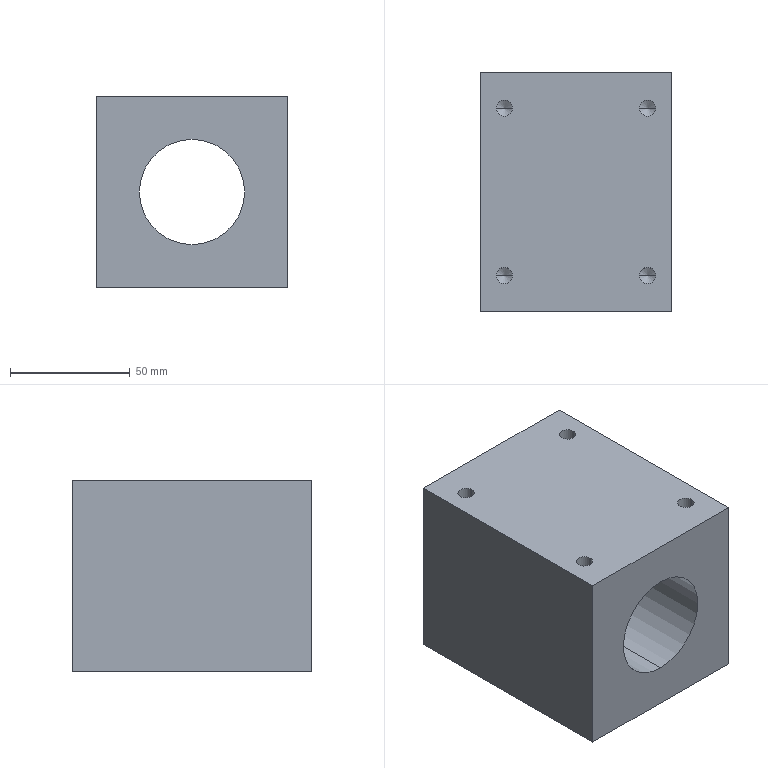Part | SolidWorks | features BaseBody 1 | 1 solid | 48 faces | box 80 x 100 x 80 mm | volume 483153 mm3 | cylinder 22 | cone 20 | plane 6 | commonest cylinder face diameters 5 x12 6.8 x8 44 x2
STEP:
#1=CARTESIAN_POINT('',(-66.6,85.,60.25));
#2=VERTEX_POINT('',#1);
#3=CARTESIAN_POINT('',(-73.4,85.,60.25));
#4=VERTEX_POINT('',#3);
#5=CARTESIAN_POINT('',(-70.,85.,60.25));
#6=DIRECTION('',(0.,0.,-1.));
#7=DIRECTION('',(1.,0.,0.));
#8=AXIS2_PLACEMENT_3D('',#5,#6,#7);
#9=CIRCLE('',#8,3.4);
#10=EDGE_CURVE('',#2,#4,#9,.T.);
#11=ORIENTED_EDGE('',*,*,#10,.T.);
#12=CARTESIAN_POINT('',(-73.4,85.,80.));
#13=VERTEX_POINT('',#12);
#14=CARTESIAN_POINT('',(-73.4,85.,60.25));
#15=DIRECTION('',(0.,0.,1.));
#16=VECTOR('',#15,1000.);
#17=LINE('',#14,#16);
#18=EDGE_CURVE('',#4,#13,#17,.T.);
#19=ORIENTED_EDGE('',*,*,#18,.T.);
#20=CARTESIAN_POINT('',(-66.6,85.,80.));
#21=VERTEX_POINT('',#20);
#22=CARTESIAN_POINT('',(-70.,85.,80.));
#23=DIRECTION('',(0.,0.,1.));
#24=DIRECTION('',(1.,0.,0.));
#25=AXIS2_PLACEMENT_3D('',#22,#23,#24);
#26=CIRCLE('',#25,3.4);
#27=EDGE_CURVE('',#13,#21,#26,.T.);
#28=ORIENTED_EDGE('',*,*,#27,.T.);
#29=CARTESIAN_POINT('',(-66.6,85.,60.25));
#30=DIRECTION('',(0.,0.,1.));
#31=VECTOR('',#30,1000.);
#32=LINE('',#29,#31);
#33=EDGE_CURVE('',#2,#21,#32,.T.);
#34=ORIENTED_EDGE('',*,*,#33,.F.);
#35=EDGE_LOOP('',(#11,#19,#28,#34));
#36=FACE_OUTER_BOUND('',#35,.T.);
#37=CARTESIAN_POINT('',(-70.,85.,60.25));
#38=DIRECTION('',(0.,0.,1.));
#39=DIRECTION('',(1.,0.,0.));
#40=AXIS2_PLACEMENT_3D('',#37,#38,#39);
#41=CYLINDRICAL_SURFACE('',#40,3.4);
#42=ADVANCED_FACE('',(#36),#41,.F.);
#43=CARTESIAN_POINT('',(-70.,85.,58.207));
#44=VERTEX_POINT('',#43);
#45=CARTESIAN_POINT('',(-70.,85.,58.207));
#46=DIRECTION('',(0.8572,0.,0.515));
#47=VECTOR('',#46,1000.);
#48=LINE('',#45,#47);
#49=EDGE_CURVE('',#44,#2,#48,.T.);
#50=ORIENTED_EDGE('',*,*,#49,.F.);
#51=CARTESIAN_POINT('',(-70.,85.,58.207));
#52=DIRECTION('',(-0.8572,0.,0.515));
#53=VECTOR('',#52,1000.);
#54=LINE('',#51,#53);
#55=EDGE_CURVE('',#44,#4,#54,.T.);
#56=ORIENTED_EDGE('',*,*,#55,.T.);
#57=ORIENTED_EDGE('',*,*,#10,.F.);
#58=EDGE_LOOP('',(#50,#56,#57));
#59=FACE_OUTER_BOUND('',#58,.T.);
#60=CARTESIAN_POINT('',(-70.,85.,1058.207));
#61=DIRECTION('',(0.,0.,1.));
#62=DIRECTION('',(1.,0.,0.));
#63=AXIS2_PLACEMENT_3D('',#60,#61,#62);
#64=CONICAL_SURFACE('',#63,1664.279,1.03);
#65=ADVANCED_FACE('',(#59),#64,.F.);
#66=CARTESIAN_POINT('',(-6.6,85.,60.25));
#67=VERTEX_POINT('',#66);
#68=CARTESIAN_POINT('',(-13.4,85.,60.25));
#69=VERTEX_POINT('',#68);
#70=CARTESIAN_POINT('',(-10.,85.,60.25));
#71=DIRECTION('',(0.,0.,-1.));
#72=DIRECTION('',(1.,0.,0.));
#73=AXIS2_PLACEMENT_3D('',#70,#71,#72);
#74=CIRCLE('',#73,3.4);
#75=EDGE_CURVE('',#67,#69,#74,.T.);
#76=ORIENTED_EDGE('',*,*,#75,.T.);
#77=CARTESIAN_POINT('',(-13.4,85.,80.));
#78=VERTEX_POINT('',#77);
#79=CARTESIAN_POINT('',(-13.4,85.,60.25));
#80=DIRECTION('',(0.,0.,1.));
#81=VECTOR('',#80,1000.);
#82=LINE('',#79,#81);
#83=EDGE_CURVE('',#69,#78,#82,.T.);
#84=ORIENTED_EDGE('',*,*,#83,.T.);
#85=CARTESIAN_POINT('',(-6.6,85.,80.));
#86=VERTEX_POINT('',#85);
#87=CARTESIAN_POINT('',(-10.,85.,80.));
#88=DIRECTION('',(0.,0.,-1.));
#89=DIRECTION('',(1.,0.,0.));
#90=AXIS2_PLACEMENT_3D('',#87,#88,#89);
#91=CIRCLE('',#90,3.4);
#92=EDGE_CURVE('',#86,#78,#91,.T.);
#93=ORIENTED_EDGE('',*,*,#92,.F.);
#94=CARTESIAN_POINT('',(-6.6,85.,60.25));
#95=DIRECTION('',(0.,0.,1.));
#96=VECTOR('',#95,1000.);
#97=LINE('',#94,#96);
#98=EDGE_CURVE('',#67,#86,#97,.T.);
#99=ORIENTED_EDGE('',*,*,#98,.F.);
#100=EDGE_LOOP('',(#76,#84,#93,#99));
#101=FACE_OUTER_BOUND('',#100,.T.);
#102=CARTESIAN_POINT('',(-10.,85.,60.25));
#103=DIRECTION('',(0.,0.,1.));
#104=DIRECTION('',(1.,0.,0.));
#105=AXIS2_PLACEMENT_3D('',#102,#103,#104);
#106=CYLINDRICAL_SURFACE('',#105,3.4);
#107=ADVANCED_FACE('',(#101),#106,.F.);
#108=CARTESIAN_POINT('',(-6.6,15.,60.25));
#109=VERTEX_POINT('',#108);
#110=CARTESIAN_POINT('',(-13.4,15.,60.25));
#111=VERTEX_POINT('',#110);
#112=CARTESIAN_POINT('',(-10.,15.,60.25));
#113=DIRECTION('',(0.,0.,-1.));
#114=DIRECTION('',(1.,0.,0.));
#115=AXIS2_PLACEMENT_3D('',#112,#113,#114);
#116=CIRCLE('',#115,3.4);
#117=EDGE_CURVE('',#109,#111,#116,.T.);
#118=ORIENTED_EDGE('',*,*,#117,.T.);
#119=CARTESIAN_POINT('',(-13.4,15.,80.));
#120=VERTEX_POINT('',#119);
#121=CARTESIAN_POINT('',(-13.4,15.,60.25));
#122=DIRECTION('',(0.,0.,1.));
#123=VECTOR('',#122,1000.);
#124=LINE('',#121,#123);
#125=EDGE_CURVE('',#111,#120,#124,.T.);
#126=ORIENTED_EDGE('',*,*,#125,.T.);
#127=CARTESIAN_POINT('',(-6.6,15.,80.));
#128=VERTEX_POINT('',#127);
#129=CARTESIAN_POINT('',(-10.,15.,80.));
#130=DIRECTION('',(0.,0.,-1.));
#131=DIRECTION('',(1.,0.,0.));
#132=AXIS2_PLACEMENT_3D('',#129,#130,#131);
#133=CIRCLE('',#132,3.4);
#134=EDGE_CURVE('',#128,#120,#133,.T.);
#135=ORIENTED_EDGE('',*,*,#134,.F.);
#136=CARTESIAN_POINT('',(-6.6,15.,60.25));
#137=DIRECTION('',(0.,0.,1.));
#138=VECTOR('',#137,1000.);
#139=LINE('',#136,#138);
#140=EDGE_CURVE('',#109,#128,#139,.T.);
#141=ORIENTED_EDGE('',*,*,#140,.F.);
#142=EDGE_LOOP('',(#118,#126,#135,#141));
#143=FACE_OUTER_BOUND('',#142,.T.);
#144=CARTESIAN_POINT('',(-10.,15.,60.25));
#145=DIRECTION('',(0.,0.,1.));
#146=DIRECTION('',(1.,0.,0.));
#147=AXIS2_PLACEMENT_3D('',#144,#145,#146);
#148=CYLINDRICAL_SURFACE('',#147,3.4);
#149=ADVANCED_FACE('',(#143),#148,.F.);
#150=CARTESIAN_POINT('',(-66.6,15.,60.25));
#151=VERTEX_POINT('',#150);
#152=CARTESIAN_POINT('',(-73.4,15.,60.25));
#153=VERTEX_POINT('',#152);
#154=CARTESIAN_POINT('',(-70.,15.,60.25));
#155=DIRECTION('',(0.,0.,-1.));
#156=DIRECTION('',(1.,0.,0.));
#157=AXIS2_PLACEMENT_3D('',#154,#155,#156);
#158=CIRCLE('',#157,3.4);
#159=EDGE_CURVE('',#151,#153,#158,.T.);
#160=ORIENTED_EDGE('',*,*,#159,.T.);
#161=CARTESIAN_POINT('',(-73.4,15.,80.));
#162=VERTEX_POINT('',#161);
#163=CARTESIAN_POINT('',(-73.4,15.,60.25));
#164=DIRECTION('',(0.,0.,1.));
#165=VECTOR('',#164,1000.);
#166=LINE('',#163,#165);
#167=EDGE_CURVE('',#153,#162,#166,.T.);
#168=ORIENTED_EDGE('',*,*,#167,.T.);
#169=CARTESIAN_POINT('',(-66.6,15.,80.));
#170=VERTEX_POINT('',#169);
#171=CARTESIAN_POINT('',(-70.,15.,80.));
#172=DIRECTION('',(0.,0.,-1.));
#173=DIRECTION('',(1.,0.,0.));
#174=AXIS2_PLACEMENT_3D('',#171,#172,#173);
#175=CIRCLE('',#174,3.4);
#176=EDGE_CURVE('',#170,#162,#175,.T.);
#177=ORIENTED_EDGE('',*,*,#176,.F.);
#178=CARTESIAN_POINT('',(-66.6,15.,60.25));
#179=DIRECTION('',(0.,0.,1.));
#180=VECTOR('',#179,1000.);
#181=LINE('',#178,#180);
#182=EDGE_CURVE('',#151,#170,#181,.T.);
#183=ORIENTED_EDGE('',*,*,#182,.F.);
#184=EDGE_LOOP('',(#160,#168,#177,#183));
#185=FACE_OUTER_BOUND('',#184,.T.);
#186=CARTESIAN_POINT('',(-70.,15.,60.25));
#187=DIRECTION('',(0.,0.,1.));
#188=DIRECTION('',(1.,0.,0.));
#189=AXIS2_PLACEMENT_3D('',#186,#187,#188);
#190=CYLINDRICAL_SURFACE('',#189,3.4);
#191=ADVANCED_FACE('',(#185),#190,.F.);
#192=CARTESIAN_POINT('',(-10.,85.,58.207));
#193=VERTEX_POINT('',#192);
#194=CARTESIAN_POINT('',(-10.,85.,58.207));
#195=DIRECTION('',(0.8572,0.,0.515));
#196=VECTOR('',#195,1000.);
#197=LINE('',#194,#196);
#198=EDGE_CURVE('',#193,#67,#197,.T.);
#199=ORIENTED_EDGE('',*,*,#198,.F.);
#200=CARTESIAN_POINT('',(-10.,85.,58.207));
#201=DIRECTION('',(-0.8572,0.,0.515));
#202=VECTOR('',#201,1000.);
#203=LINE('',#200,#202);
#204=EDGE_CURVE('',#193,#69,#203,.T.);
#205=ORIENTED_EDGE('',*,*,#204,.T.);
#206=ORIENTED_EDGE('',*,*,#75,.F.);
#207=EDGE_LOOP('',(#199,#205,#206));
#208=FACE_OUTER_BOUND('',#207,.T.);
#209=CARTESIAN_POINT('',(-10.,85.,1058.207));
#210=DIRECTION('',(0.,0.,1.));
#211=DIRECTION('',(1.,0.,0.));
#212=AXIS2_PLACEMENT_3D('',#209,#210,#211);
#213=CONICAL_SURFACE('',#212,1664.279,1.03);
#214=ADVANCED_FACE('',(#208),#213,.F.);
#215=CARTESIAN_POINT('',(-10.,15.,58.207));
#216=VERTEX_POINT('',#215);
#217=CARTESIAN_POINT('',(-10.,15.,58.207));
#218=DIRECTION('',(0.8572,0.,0.515));
#219=VECTOR('',#218,1000.);
#220=LINE('',#217,#219);
#221=EDGE_CURVE('',#216,#109,#220,.T.);
#222=ORIENTED_EDGE('',*,*,#221,.F.);
#223=CARTESIAN_POINT('',(-10.,15.,58.207));
#224=DIRECTION('',(-0.8572,0.,0.515));
#225=VECTOR('',#224,1000.);
#226=LINE('',#223,#225);
#227=EDGE_CURVE('',#216,#111,#226,.T.);
#228=ORIENTED_EDGE('',*,*,#227,.T.);
#229=ORIENTED_EDGE('',*,*,#117,.F.);
#230=EDGE_LOOP('',(#222,#228,#229));
#231=FACE_OUTER_BOUND('',#230,.T.);
#232=CARTESIAN_POINT('',(-10.,15.,1058.207));
#233=DIRECTION('',(0.,0.,1.));
#234=DIRECTION('',(1.,0.,0.));
#235=AXIS2_PLACEMENT_3D('',#232,#233,#234);
#236=CONICAL_SURFACE('',#235,1664.279,1.03);
#237=ADVANCED_FACE('',(#231),#236,.F.);
#238=CARTESIAN_POINT('',(-70.,15.,58.207));
#239=VERTEX_POINT('',#238);
#240=CARTESIAN_POINT('',(-70.,15.,58.207));
#241=DIRECTION('',(0.8572,0.,0.515));
#242=VECTOR('',#241,1000.);
#243=LINE('',#240,#242);
#244=EDGE_CURVE('',#239,#151,#243,.T.);
#245=ORIENTED_EDGE('',*,*,#244,.F.);
#246=CARTESIAN_POINT('',(-70.,15.,58.207));
#247=DIRECTION('',(-0.8572,0.,0.515));
#248=VECTOR('',#247,1000.);
#249=LINE('',#246,#248);
#250=EDGE_CURVE('',#239,#153,#249,.T.);
#251=ORIENTED_EDGE('',*,*,#250,.T.);
#252=ORIENTED_EDGE('',*,*,#159,.F.);
#253=EDGE_LOOP('',(#245,#251,#252));
#254=FACE_OUTER_BOUND('',#253,.T.);
#255=CARTESIAN_POINT('',(-70.,15.,1058.207));
#256=DIRECTION('',(0.,0.,1.));
#257=DIRECTION('',(1.,0.,0.));
#258=AXIS2_PLACEMENT_3D('',#255,#256,#257);
#259=CONICAL_SURFACE('',#258,1664.279,1.03);
#260=ADVANCED_FACE('',(#254),#259,.F.);
#261=CARTESIAN_POINT('',(-15.751,85.,28.5));
#262=VERTEX_POINT('',#261);
#263=CARTESIAN_POINT('',(-15.751,85.,23.5));
#264=VERTEX_POINT('',#263);
#265=CARTESIAN_POINT('',(-15.751,85.,26.));
#266=DIRECTION('',(0.,-1.,0.));
#267=DIRECTION('',(0.,0.,1.));
#268=AXIS2_PLACEMENT_3D('',#265,#266,#267);
#269=CIRCLE('',#268,2.5);
#270=EDGE_CURVE('',#262,#264,#269,.T.);
#271=ORIENTED_EDGE('',*,*,#270,.T.);
#272=CARTESIAN_POINT('',(-15.751,100.,23.5));
#273=VERTEX_POINT('',#272);
#274=CARTESIAN_POINT('',(-15.751,85.,23.5));
#275=DIRECTION('',(0.,1.,0.));
#276=VECTOR('',#275,1000.);
#277=LINE('',#274,#276);
#278=EDGE_CURVE('',#264,#273,#277,.T.);
#279=ORIENTED_EDGE('',*,*,#278,.T.);
#280=CARTESIAN_POINT('',(-15.751,100.,28.5));
#281=VERTEX_POINT('',#280);
#282=CARTESIAN_POINT('',(-15.751,100.,26.));
#283=DIRECTION('',(0.,1.,0.));
#284=DIRECTION('',(0.,0.,1.));
#285=AXIS2_PLACEMENT_3D('',#282,#283,#284);
#286=CIRCLE('',#285,2.5);
#287=EDGE_CURVE('',#273,#281,#286,.T.);
#288=ORIENTED_EDGE('',*,*,#287,.T.);
#289=CARTESIAN_POINT('',(-15.751,85.,28.5));
#290=DIRECTION('',(0.,1.,0.));
#291=VECTOR('',#290,1000.);
#292=LINE('',#289,#291);
#293=EDGE_CURVE('',#262,#281,#292,.T.);
#294=ORIENTED_EDGE('',*,*,#293,.F.);
#295=EDGE_LOOP('',(#271,#279,#288,#294));
#296=FACE_OUTER_BOUND('',#295,.T.);
#297=CARTESIAN_POINT('',(-15.751,85.,26.));
#298=DIRECTION('',(0.,1.,0.));
#299=DIRECTION('',(0.,0.,1.));
#300=AXIS2_PLACEMENT_3D('',#297,#298,#299);
#301=CYLINDRICAL_SURFACE('',#300,2.5);
#302=ADVANCED_FACE('',(#296),#301,.F.);
#303=CARTESIAN_POINT('',(-15.751,85.,56.5));
#304=VERTEX_POINT('',#303);
#305=CARTESIAN_POINT('',(-15.751,85.,51.5));
#306=VERTEX_POINT('',#305);
#307=CARTESIAN_POINT('',(-15.751,85.,54.));
#308=DIRECTION('',(0.,-1.,0.));
#309=DIRECTION('',(0.,0.,1.));
#310=AXIS2_PLACEMENT_3D('',#307,#308,#309);
#311=CIRCLE('',#310,2.5);
#312=EDGE_CURVE('',#304,#306,#311,.T.);
#313=ORIENTED_EDGE('',*,*,#312,.T.);
#314=CARTESIAN_POINT('',(-15.751,100.,51.5));
#315=VERTEX_POINT('',#314);
#316=CARTESIAN_POINT('',(-15.751,85.,51.5));
#317=DIRECTION('',(0.,1.,0.));
#318=VECTOR('',#317,1000.);
#319=LINE('',#316,#318);
#320=EDGE_CURVE('',#306,#315,#319,.T.);
#321=ORIENTED_EDGE('',*,*,#320,.T.);
#322=CARTESIAN_POINT('',(-15.751,100.,56.5));
#323=VERTEX_POINT('',#322);
#324=CARTESIAN_POINT('',(-15.751,100.,54.));
#325=DIRECTION('',(0.,1.,0.));
#326=DIRECTION('',(0.,0.,1.));
#327=AXIS2_PLACEMENT_3D('',#324,#325,#326);
#328=CIRCLE('',#327,2.5);
#329=EDGE_CURVE('',#315,#323,#328,.T.);
#330=ORIENTED_EDGE('',*,*,#329,.T.);
#331=CARTESIAN_POINT('',(-15.751,85.,56.5));
#332=DIRECTION('',(0.,1.,0.));
#333=VECTOR('',#332,1000.);
#334=LINE('',#331,#333);
#335=EDGE_CURVE('',#304,#323,#334,.T.);
#336=ORIENTED_EDGE('',*,*,#335,.F.);
#337=EDGE_LOOP('',(#313,#321,#330,#336));
#338=FACE_OUTER_BOUND('',#337,.T.);
#339=CARTESIAN_POINT('',(-15.751,85.,54.));
#340=DIRECTION('',(0.,1.,0.));
#341=DIRECTION('',(0.,0.,1.));
#342=AXIS2_PLACEMENT_3D('',#339,#340,#341);
#343=CYLINDRICAL_SURFACE('',#342,2.5);
#344=ADVANCED_FACE('',(#338),#343,.F.);
#345=CARTESIAN_POINT('',(-40.,85.,70.5));
#346=VERTEX_POINT('',#345);
#347=CARTESIAN_POINT('',(-40.,85.,65.5));
#348=VERTEX_POINT('',#347);
#349=CARTESIAN_POINT('',(-40.,85.,68.));
#350=DIRECTION('',(0.,-1.,0.));
#351=DIRECTION('',(0.,0.,1.));
#352=AXIS2_PLACEMENT_3D('',#349,#350,#351);
#353=CIRCLE('',#352,2.5);
#354=EDGE_CURVE('',#346,#348,#353,.T.);
#355=ORIENTED_EDGE('',*,*,#354,.T.);
#356=CARTESIAN_POINT('',(-40.,100.,65.5));
#357=VERTEX_POINT('',#356);
#358=CARTESIAN_POINT('',(-40.,85.,65.5));
#359=DIRECTION('',(0.,1.,0.));
#360=VECTOR('',#359,1000.);
#361=LINE('',#358,#360);
#362=EDGE_CURVE('',#348,#357,#361,.T.);
#363=ORIENTED_EDGE('',*,*,#362,.T.);
#364=CARTESIAN_POINT('',(-40.,100.,70.5));
#365=VERTEX_POINT('',#364);
#366=CARTESIAN_POINT('',(-40.,100.,68.));
#367=DIRECTION('',(0.,1.,0.));
#368=DIRECTION('',(0.,0.,1.));
#369=AXIS2_PLACEMENT_3D('',#366,#367,#368);
#370=CIRCLE('',#369,2.5);
#371=EDGE_CURVE('',#357,#365,#370,.T.);
#372=ORIENTED_EDGE('',*,*,#371,.T.);
#373=CARTESIAN_POINT('',(-40.,85.,70.5));
#374=DIRECTION('',(0.,1.,0.));
#375=VECTOR('',#374,1000.);
#376=LINE('',#373,#375);
#377=EDGE_CURVE('',#346,#365,#376,.T.);
#378=ORIENTED_EDGE('',*,*,#377,.F.);
#379=EDGE_LOOP('',(#355,#363,#372,#378));
#380=FACE_OUTER_BOUND('',#379,.T.);
#381=CARTESIAN_POINT('',(-40.,85.,68.));
#382=DIRECTION('',(0.,1.,0.));
#383=DIRECTION('',(0.,0.,1.));
#384=AXIS2_PLACEMENT_3D('',#381,#382,#383);
#385=CYLINDRICAL_SURFACE('',#384,2.5);
#386=ADVANCED_FACE('',(#380),#385,.F.);
#387=CARTESIAN_POINT('',(-64.249,85.,56.5));
#388=VERTEX_POINT('',#387);
#389=CARTESIAN_POINT('',(-64.249,85.,51.5));
#390=VERTEX_POINT('',#389);
#391=CARTESIAN_POINT('',(-64.249,85.,54.));
#392=DIRECTION('',(0.,-1.,0.));
#393=DIRECTION('',(0.,0.,1.));
#394=AXIS2_PLACEMENT_3D('',#391,#392,#393);
#395=CIRCLE('',#394,2.5);
#396=EDGE_CURVE('',#388,#390,#395,.T.);
#397=ORIENTED_EDGE('',*,*,#396,.T.);
#398=CARTESIAN_POINT('',(-64.249,100.,51.5));
#399=VERTEX_POINT('',#398);
#400=CARTESIAN_POINT('',(-64.249,85.,51.5));
#401=DIRECTION('',(0.,1.,0.));
#402=VECTOR('',#401,1000.);
#403=LINE('',#400,#402);
#404=EDGE_CURVE('',#390,#399,#403,.T.);
#405=ORIENTED_EDGE('',*,*,#404,.T.);
#406=CARTESIAN_POINT('',(-64.249,100.,56.5));
#407=VERTEX_POINT('',#406);
#408=CARTESIAN_POINT('',(-64.249,100.,54.));
#409=DIRECTION('',(0.,1.,0.));
#410=DIRECTION('',(0.,0.,1.));
#411=AXIS2_PLACEMENT_3D('',#408,#409,#410);
#412=CIRCLE('',#411,2.5);
#413=EDGE_CURVE('',#399,#407,#412,.T.);
#414=ORIENTED_EDGE('',*,*,#413,.T.);
#415=CARTESIAN_POINT('',(-64.249,85.,56.5));
#416=DIRECTION('',(0.,1.,0.));
#417=VECTOR('',#416,1000.);
#418=LINE('',#415,#417);
#419=EDGE_CURVE('',#388,#407,#418,.T.);
#420=ORIENTED_EDGE('',*,*,#419,.F.);
#421=EDGE_LOOP('',(#397,#405,#414,#420));
#422=FACE_OUTER_BOUND('',#421,.T.);
#423=CARTESIAN_POINT('',(-64.249,85.,54.));
#424=DIRECTION('',(0.,1.,0.));
#425=DIRECTION('',(0.,0.,1.));
#426=AXIS2_PLACEMENT_3D('',#423,#424,#425);
#427=CYLINDRICAL_SURFACE('',#426,2.5);
#428=ADVANCED_FACE('',(#422),#427,.F.);
#429=CARTESIAN_POINT('',(-64.249,85.,28.5));
#430=VERTEX_POINT('',#429);
#431=CARTESIAN_POINT('',(-64.249,85.,23.5));
#432=VERTEX_POINT('',#431);
#433=CARTESIAN_POINT('',(-64.249,85.,26.));
#434=DIRECTION('',(0.,-1.,0.));
#435=DIRECTION('',(0.,0.,1.));
#436=AXIS2_PLACEMENT_3D('',#433,#434,#435);
#437=CIRCLE('',#436,2.5);
#438=EDGE_CURVE('',#430,#432,#437,.T.);
#439=ORIENTED_EDGE('',*,*,#438,.T.);
#440=CARTESIAN_POINT('',(-64.249,100.,23.5));
#441=VERTEX_POINT('',#440);
#442=CARTESIAN_POINT('',(-64.249,85.,23.5));
#443=DIRECTION('',(0.,1.,0.));
#444=VECTOR('',#443,1000.);
#445=LINE('',#442,#444);
#446=EDGE_CURVE('',#432,#441,#445,.T.);
#447=ORIENTED_EDGE('',*,*,#446,.T.);
#448=CARTESIAN_POINT('',(-64.249,100.,28.5));
#449=VERTEX_POINT('',#448);
#450=CARTESIAN_POINT('',(-64.249,100.,26.));
#451=DIRECTION('',(0.,1.,0.));
#452=DIRECTION('',(0.,0.,1.));
#453=AXIS2_PLACEMENT_3D('',#450,#451,#452);
#454=CIRCLE('',#453,2.5);
#455=EDGE_CURVE('',#441,#449,#454,.T.);
#456=ORIENTED_EDGE('',*,*,#455,.T.);
#457=CARTESIAN_POINT('',(-64.249,85.,28.5));
#458=DIRECTION('',(0.,1.,0.));
#459=VECTOR('',#458,1000.);
#460=LINE('',#457,#459);
#461=EDGE_CURVE('',#430,#449,#460,.T.);
#462=ORIENTED_EDGE('',*,*,#461,.F.);
#463=EDGE_LOOP('',(#439,#447,#456,#462));
#464=FACE_OUTER_BOUND('',#463,.T.);
#465=CARTESIAN_POINT('',(-64.249,85.,26.));
#466=DIRECTION('',(0.,1.,0.));
#467=DIRECTION('',(0.,0.,1.));
#468=AXIS2_PLACEMENT_3D('',#465,#466,#467);
#469=CYLINDRICAL_SURFACE('',#468,2.5);
#470=ADVANCED_FACE('',(#464),#469,.F.);
#471=CARTESIAN_POINT('',(-40.,85.,14.5));
#472=VERTEX_POINT('',#471);
#473=CARTESIAN_POINT('',(-40.,85.,9.5));
#474=VERTEX_POINT('',#473);
#475=CARTESIAN_POINT('',(-40.,85.,12.));
#476=DIRECTION('',(0.,-1.,0.));
#477=DIRECTION('',(0.,0.,1.));
#478=AXIS2_PLACEMENT_3D('',#475,#476,#477);
#479=CIRCLE('',#478,2.5);
#480=EDGE_CURVE('',#472,#474,#479,.T.);
#481=ORIENTED_EDGE('',*,*,#480,.T.);
#482=CARTESIAN_POINT('',(-40.,100.,9.5));
#483=VERTEX_POINT('',#482);
#484=CARTESIAN_POINT('',(-40.,85.,9.5));
#485=DIRECTION('',(0.,1.,0.));
#486=VECTOR('',#485,1000.);
#487=LINE('',#484,#486);
#488=EDGE_CURVE('',#474,#483,#487,.T.);
#489=ORIENTED_EDGE('',*,*,#488,.T.);
#490=CARTESIAN_POINT('',(-40.,100.,14.5));
#491=VERTEX_POINT('',#490);
#492=CARTESIAN_POINT('',(-40.,100.,12.));
#493=DIRECTION('',(0.,1.,0.));
#494=DIRECTION('',(0.,0.,1.));
#495=AXIS2_PLACEMENT_3D('',#492,#493,#494);
#496=CIRCLE('',#495,2.5);
#497=EDGE_CURVE('',#483,#491,#496,.T.);
#498=ORIENTED_EDGE('',*,*,#497,.T.);
#499=CARTESIAN_POINT('',(-40.,85.,14.5));
#500=DIRECTION('',(0.,1.,0.));
#501=VECTOR('',#500,1000.);
#502=LINE('',#499,#501);
#503=EDGE_CURVE('',#472,#491,#502,.T.);
#504=ORIENTED_EDGE('',*,*,#503,.F.);
#505=EDGE_LOOP('',(#481,#489,#498,#504));
#506=FACE_OUTER_BOUND('',#505,.T.);
#507=CARTESIAN_POINT('',(-40.,85.,12.));
#508=DIRECTION('',(0.,1.,0.));
#509=DIRECTION('',(0.,0.,1.));
#510=AXIS2_PLACEMENT_3D('',#507,#508,#509);
#511=CYLINDRICAL_SURFACE('',#510,2.5);
#512=ADVANCED_FACE('',(#506),#511,.F.);
#513=CARTESIAN_POINT('',(-40.,0.,62.));
#514=VERTEX_POINT('',#513);
#515=CARTESIAN_POINT('',(-40.,0.,18.));
#516=VERTEX_POINT('',#515);
#517=CARTESIAN_POINT('',(-40.,0.,40.));
#518=DIRECTION('',(0.,-1.,0.));
#519=DIRECTION('',(0.,0.,1.));
#520=AXIS2_PLACEMENT_3D('',#517,#518,#519);
#521=CIRCLE('',#520,22.);
#522=EDGE_CURVE('',#514,#516,#521,.T.);
#523=ORIENTED_EDGE('',*,*,#522,.T.);
#524=CARTESIAN_POINT('',(-40.,100.,18.));
#525=VERTEX_POINT('',#524);
#526=CARTESIAN_POINT('',(-40.,0.,18.));
#527=DIRECTION('',(0.,1.,0.));
#528=VECTOR('',#527,1000.);
#529=LINE('',#526,#528);
#530=EDGE_CURVE('',#516,#525,#529,.T.);
#531=ORIENTED_EDGE('',*,*,#530,.T.);
#532=CARTESIAN_POINT('',(-40.,100.,62.));
#533=VERTEX_POINT('',#532);
#534=CARTESIAN_POINT('',(-40.,100.,40.));
#535=DIRECTION('',(0.,1.,0.));
#536=DIRECTION('',(0.,0.,1.));
#537=AXIS2_PLACEMENT_3D('',#534,#535,#536);
#538=CIRCLE('',#537,22.);
#539=EDGE_CURVE('',#525,#533,#538,.T.);
#540=ORIENTED_EDGE('',*,*,#539,.T.);
#541=CARTESIAN_POINT('',(-40.,0.,62.));
#542=DIRECTION('',(0.,1.,0.));
#543=VECTOR('',#542,1000.);
#544=LINE('',#541,#543);
#545=EDGE_CURVE('',#514,#533,#544,.T.);
#546=ORIENTED_EDGE('',*,*,#545,.F.);
#547=EDGE_LOOP('',(#523,#531,#540,#546));
#548=FACE_OUTER_BOUND('',#547,.T.);
#549=CARTESIAN_POINT('',(-40.,0.,40.));
#550=DIRECTION('',(0.,1.,0.));
#551=DIRECTION('',(0.,0.,1.));
#552=AXIS2_PLACEMENT_3D('',#549,#550,#551);
#553=CYLINDRICAL_SURFACE('',#552,22.);
#554=ADVANCED_FACE('',(#548),#553,.F.);
#555=CARTESIAN_POINT('',(-15.751,83.498,26.));
#556=VERTEX_POINT('',#555);
#557=CARTESIAN_POINT('',(-15.751,83.498,26.));
#558=DIRECTION('',(0.,0.515,0.8572));
#559=VECTOR('',#558,1000.);
#560=LINE('',#557,#559);
#561=EDGE_CURVE('',#556,#262,#560,.T.);
#562=ORIENTED_EDGE('',*,*,#561,.F.);
#563=CARTESIAN_POINT('',(-15.751,83.498,26.));
#564=DIRECTION('',(0.,0.515,-0.8572));
#565=VECTOR('',#564,1000.);
#566=LINE('',#563,#565);
#567=EDGE_CURVE('',#556,#264,#566,.T.);
#568=ORIENTED_EDGE('',*,*,#567,.T.);
#569=ORIENTED_EDGE('',*,*,#270,.F.);
#570=EDGE_LOOP('',(#562,#568,#569));
#571=FACE_OUTER_BOUND('',#570,.T.);
#572=CARTESIAN_POINT('',(-15.751,1083.498,26.));
#573=DIRECTION('',(0.,1.,0.));
#574=DIRECTION('',(0.,0.,1.));
#575=AXIS2_PLACEMENT_3D('',#572,#573,#574);
#576=CONICAL_SURFACE('',#575,1664.279,1.03);
#577=ADVANCED_FACE('',(#571),#576,.F.);
#578=CARTESIAN_POINT('',(-15.751,83.498,54.));
#579=VERTEX_POINT('',#578);
#580=CARTESIAN_POINT('',(-15.751,83.498,54.));
#581=DIRECTION('',(0.,0.515,0.8572));
#582=VECTOR('',#581,1000.);
#583=LINE('',#580,#582);
#584=EDGE_CURVE('',#579,#304,#583,.T.);
#585=ORIENTED_EDGE('',*,*,#584,.F.);
#586=CARTESIAN_POINT('',(-15.751,83.498,54.));
#587=DIRECTION('',(0.,0.515,-0.8572));
#588=VECTOR('',#587,1000.);
#589=LINE('',#586,#588);
#590=EDGE_CURVE('',#579,#306,#589,.T.);
#591=ORIENTED_EDGE('',*,*,#590,.T.);
#592=ORIENTED_EDGE('',*,*,#312,.F.);
#593=EDGE_LOOP('',(#585,#591,#592));
#594=FACE_OUTER_BOUND('',#593,.T.);
#595=CARTESIAN_POINT('',(-15.751,1083.498,54.));
#596=DIRECTION('',(0.,1.,0.));
#597=DIRECTION('',(0.,0.,1.));
#598=AXIS2_PLACEMENT_3D('',#595,#596,#597);
#599=CONICAL_SURFACE('',#598,1664.279,1.03);
#600=ADVANCED_FACE('',(#594),#599,.F.);
#601=CARTESIAN_POINT('',(-40.,83.498,68.));
#602=VERTEX_POINT('',#601);
#603=CARTESIAN_POINT('',(-40.,83.498,68.));
#604=DIRECTION('',(0.,0.515,0.8572));
#605=VECTOR('',#604,1000.);
#606=LINE('',#603,#605);
#607=EDGE_CURVE('',#602,#346,#606,.T.);
#608=ORIENTED_EDGE('',*,*,#607,.F.);
#609=CARTESIAN_POINT('',(-40.,83.498,68.));
#610=DIRECTION('',(0.,0.515,-0.8572));
#611=VECTOR('',#610,1000.);
#612=LINE('',#609,#611);
#613=EDGE_CURVE('',#602,#348,#612,.T.);
#614=ORIENTED_EDGE('',*,*,#613,.T.);
#615=ORIENTED_EDGE('',*,*,#354,.F.);
#616=EDGE_LOOP('',(#608,#614,#615));
#617=FACE_OUTER_BOUND('',#616,.T.);
#618=CARTESIAN_POINT('',(-40.,1083.498,68.));
#619=DIRECTION('',(0.,1.,0.));
#620=DIRECTION('',(0.,0.,1.));
#621=AXIS2_PLACEMENT_3D('',#618,#619,#620);
#622=CONICAL_SURFACE('',#621,1664.279,1.03);
#623=ADVANCED_FACE('',(#617),#622,.F.);
#624=CARTESIAN_POINT('',(-64.249,83.498,54.));
#625=VERTEX_POINT('',#624);
#626=CARTESIAN_POINT('',(-64.249,83.498,54.));
#627=DIRECTION('',(0.,0.515,0.8572));
#628=VECTOR('',#627,1000.);
#629=LINE('',#626,#628);
#630=EDGE_CURVE('',#625,#388,#629,.T.);
#631=ORIENTED_EDGE('',*,*,#630,.F.);
#632=CARTESIAN_POINT('',(-64.249,83.498,54.));
#633=DIRECTION('',(0.,0.515,-0.8572));
#634=VECTOR('',#633,1000.);
#635=LINE('',#632,#634);
#636=EDGE_CURVE('',#625,#390,#635,.T.);
#637=ORIENTED_EDGE('',*,*,#636,.T.);
#638=ORIENTED_EDGE('',*,*,#396,.F.);
#639=EDGE_LOOP('',(#631,#637,#638));
#640=FACE_OUTER_BOUND('',#639,.T.);
#641=CARTESIAN_POINT('',(-64.249,1083.498,54.));
#642=DIRECTION('',(0.,1.,0.));
#643=DIRECTION('',(0.,0.,1.));
#644=AXIS2_PLACEMENT_3D('',#641,#642,#643);
#645=CONICAL_SURFACE('',#644,1664.279,1.03);
#646=ADVANCED_FACE('',(#640),#645,.F.);
#647=CARTESIAN_POINT('',(-64.249,83.498,26.));
#648=VERTEX_POINT('',#647);
#649=CARTESIAN_POINT('',(-64.249,83.498,26.));
#650=DIRECTION('',(0.,0.515,0.8572));
#651=VECTOR('',#650,1000.);
#652=LINE('',#649,#651);
#653=EDGE_CURVE('',#648,#430,#652,.T.);
#654=ORIENTED_EDGE('',*,*,#653,.F.);
#655=CARTESIAN_POINT('',(-64.249,83.498,26.));
#656=DIRECTION('',(0.,0.515,-0.8572));
#657=VECTOR('',#656,1000.);
#658=LINE('',#655,#657);
#659=EDGE_CURVE('',#648,#432,#658,.T.);
#660=ORIENTED_EDGE('',*,*,#659,.T.);
#661=ORIENTED_EDGE('',*,*,#438,.F.);
#662=EDGE_LOOP('',(#654,#660,#661));
#663=FACE_OUTER_BOUND('',#662,.T.);
#664=CARTESIAN_POINT('',(-64.249,1083.498,26.));
#665=DIRECTION('',(0.,1.,0.));
#666=DIRECTION('',(0.,0.,1.));
#667=AXIS2_PLACEMENT_3D('',#664,#665,#666);
#668=CONICAL_SURFACE('',#667,1664.279,1.03);
#669=ADVANCED_FACE('',(#663),#668,.F.);
#670=CARTESIAN_POINT('',(-40.,83.498,12.));
#671=VERTEX_POINT('',#670);
#672=CARTESIAN_POINT('',(-40.,83.498,12.));
#673=DIRECTION('',(0.,0.515,0.8572));
#674=VECTOR('',#673,1000.);
#675=LINE('',#672,#674);
#676=EDGE_CURVE('',#671,#472,#675,.T.);
#677=ORIENTED_EDGE('',*,*,#676,.F.);
#678=CARTESIAN_POINT('',(-40.,83.498,12.));
#679=DIRECTION('',(0.,0.515,-0.8572));
#680=VECTOR('',#679,1000.);
#681=LINE('',#678,#680);
#682=EDGE_CURVE('',#671,#474,#681,.T.);
#683=ORIENTED_EDGE('',*,*,#682,.T.);
#684=ORIENTED_EDGE('',*,*,#480,.F.);
#685=EDGE_LOOP('',(#677,#683,#684));
#686=FACE_OUTER_BOUND('',#685,.T.);
#687=CARTESIAN_POINT('',(-40.,1083.498,12.));
#688=DIRECTION('',(0.,1.,0.));
#689=DIRECTION('',(0.,0.,1.));
#690=AXIS2_PLACEMENT_3D('',#687,#688,#689);
#691=CONICAL_SURFACE('',#690,1664.279,1.03);
#692=ADVANCED_FACE('',(#686),#691,.F.);
#693=ORIENTED_EDGE('',*,*,#18,.F.);
#694=CARTESIAN_POINT('',(-70.,85.,60.25));
#695=DIRECTION('',(0.,0.,-1.));
#696=DIRECTION('',(1.,0.,0.));
#697=AXIS2_PLACEMENT_3D('',#694,#695,#696);
#698=CIRCLE('',#697,3.4);
#699=EDGE_CURVE('',#4,#2,#698,.T.);
#700=ORIENTED_EDGE('',*,*,#699,.T.);
#701=ORIENTED_EDGE('',*,*,#33,.T.);
#702=CARTESIAN_POINT('',(-70.,85.,80.));
#703=DIRECTION('',(0.,0.,1.));
#704=DIRECTION('',(1.,0.,0.));
#705=AXIS2_PLACEMENT_3D('',#702,#703,#704);
#706=CIRCLE('',#705,3.4);
#707=EDGE_CURVE('',#21,#13,#706,.T.);
#708=ORIENTED_EDGE('',*,*,#707,.T.);
#709=EDGE_LOOP('',(#693,#700,#701,#708));
#710=FACE_OUTER_BOUND('',#709,.T.);
#711=CARTESIAN_POINT('',(-70.,85.,60.25));
#712=DIRECTION('',(0.,0.,1.));
#713=DIRECTION('',(1.,0.,0.));
#714=AXIS2_PLACEMENT_3D('',#711,#712,#713);
#715=CYLINDRICAL_SURFACE('',#714,3.4);
#716=ADVANCED_FACE('',(#710),#715,.F.);
#717=ORIENTED_EDGE('',*,*,#92,.T.);
#718=CARTESIAN_POINT('',(-10.,85.,80.));
#719=DIRECTION('',(0.,0.,-1.));
#720=DIRECTION('',(1.,0.,0.));
#721=AXIS2_PLACEMENT_3D('',#718,#719,#720);
#722=CIRCLE('',#721,3.4);
#723=EDGE_CURVE('',#78,#86,#722,.T.);
#724=ORIENTED_EDGE('',*,*,#723,.T.);
#725=EDGE_LOOP('',(#717,#724));
#726=FACE_BOUND('',#725,.T.);
#727=ORIENTED_EDGE('',*,*,#134,.T.);
#728=CARTESIAN_POINT('',(-10.,15.,80.));
#729=DIRECTION('',(0.,0.,-1.));
#730=DIRECTION('',(1.,0.,0.));
#731=AXIS2_PLACEMENT_3D('',#728,#729,#730);
#732=CIRCLE('',#731,3.4);
#733=EDGE_CURVE('',#120,#128,#732,.T.);
#734=ORIENTED_EDGE('',*,*,#733,.T.);
#735=EDGE_LOOP('',(#727,#734));
#736=FACE_BOUND('',#735,.T.);
#737=ORIENTED_EDGE('',*,*,#176,.T.);
#738=CARTESIAN_POINT('',(-70.,15.,80.));
#739=DIRECTION('',(0.,0.,-1.));
#740=DIRECTION('',(1.,0.,0.));
#741=AXIS2_PLACEMENT_3D('',#738,#739,#740);
#742=CIRCLE('',#741,3.4);
#743=EDGE_CURVE('',#162,#170,#742,.T.);
#744=ORIENTED_EDGE('',*,*,#743,.T.);
#745=EDGE_LOOP('',(#737,#744));
#746=FACE_BOUND('',#745,.T.);
#747=ORIENTED_EDGE('',*,*,#707,.F.);
#748=ORIENTED_EDGE('',*,*,#27,.F.);
#749=EDGE_LOOP('',(#747,#748));
#750=FACE_BOUND('',#749,.T.);
#751=CARTESIAN_POINT('',(0.,0.,80.));
#752=VERTEX_POINT('',#751);
#753=CARTESIAN_POINT('',(0.,100.,80.));
#754=VERTEX_POINT('',#753);
#755=CARTESIAN_POINT('',(0.,50.,80.));
#756=DIRECTION('',(0.,1.,0.));
#757=VECTOR('',#756,1000.);
#758=LINE('',#755,#757);
#759=EDGE_CURVE('',#752,#754,#758,.T.);
#760=ORIENTED_EDGE('',*,*,#759,.T.);
#761=CARTESIAN_POINT('',(-80.,100.,80.));
#762=VERTEX_POINT('',#761);
#763=CARTESIAN_POINT('',(-40.,100.,80.));
#764=DIRECTION('',(-1.,0.,0.));
#765=VECTOR('',#764,1000.);
#766=LINE('',#763,#765);
#767=EDGE_CURVE('',#754,#762,#766,.T.);
#768=ORIENTED_EDGE('',*,*,#767,.T.);
#769=CARTESIAN_POINT('',(-80.,0.,80.));
#770=VERTEX_POINT('',#769);
#771=CARTESIAN_POINT('',(-80.,50.,80.));
#772=DIRECTION('',(0.,-1.,0.));
#773=VECTOR('',#772,1000.);
#774=LINE('',#771,#773);
#775=EDGE_CURVE('',#762,#770,#774,.T.);
#776=ORIENTED_EDGE('',*,*,#775,.T.);
#777=CARTESIAN_POINT('',(-40.,0.,80.));
#778=DIRECTION('',(1.,0.,0.));
#779=VECTOR('',#778,1000.);
#780=LINE('',#777,#779);
#781=EDGE_CURVE('',#770,#752,#780,.T.);
#782=ORIENTED_EDGE('',*,*,#781,.T.);
#783=EDGE_LOOP('',(#760,#768,#776,#782));
#784=FACE_OUTER_BOUND('',#783,.T.);
#785=CARTESIAN_POINT('',(-80.,0.,80.));
#786=DIRECTION('',(0.,0.,1.));
#787=DIRECTION('',(1.,0.,0.));
#788=AXIS2_PLACEMENT_3D('',#785,#786,#787);
#789=PLANE('',#788);
#790=ADVANCED_FACE('',(#726,#736,#746,#750,#784),#789,.T.);
#791=ORIENTED_EDGE('',*,*,#55,.F.);
#792=ORIENTED_EDGE('',*,*,#49,.T.);
#793=ORIENTED_EDGE('',*,*,#699,.F.);
#794=EDGE_LOOP('',(#791,#792,#793));
#795=FACE_OUTER_BOUND('',#794,.T.);
#796=CARTESIAN_POINT('',(-70.,85.,1058.207));
#797=DIRECTION('',(0.,0.,1.));
#798=DIRECTION('',(1.,0.,0.));
#799=AXIS2_PLACEMENT_3D('',#796,#797,#798);
#800=CONICAL_SURFACE('',#799,1664.279,1.03);
#801=ADVANCED_FACE('',(#795),#800,.F.);
#802=ORIENTED_EDGE('',*,*,#83,.F.);
#803=CARTESIAN_POINT('',(-10.,85.,60.25));
#804=DIRECTION('',(0.,0.,-1.));
#805=DIRECTION('',(1.,0.,0.));
#806=AXIS2_PLACEMENT_3D('',#803,#804,#805);
#807=CIRCLE('',#806,3.4);
#808=EDGE_CURVE('',#69,#67,#807,.T.);
#809=ORIENTED_EDGE('',*,*,#808,.T.);
#810=ORIENTED_EDGE('',*,*,#98,.T.);
#811=ORIENTED_EDGE('',*,*,#723,.F.);
#812=EDGE_LOOP('',(#802,#809,#810,#811));
#813=FACE_OUTER_BOUND('',#812,.T.);
#814=CARTESIAN_POINT('',(-10.,85.,60.25));
#815=DIRECTION('',(0.,0.,1.));
#816=DIRECTION('',(1.,0.,0.));
#817=AXIS2_PLACEMENT_3D('',#814,#815,#816);
#818=CYLINDRICAL_SURFACE('',#817,3.4);
#819=ADVANCED_FACE('',(#813),#818,.F.);
#820=ORIENTED_EDGE('',*,*,#125,.F.);
#821=CARTESIAN_POINT('',(-10.,15.,60.25));
#822=DIRECTION('',(0.,0.,-1.));
#823=DIRECTION('',(1.,0.,0.));
#824=AXIS2_PLACEMENT_3D('',#821,#822,#823);
#825=CIRCLE('',#824,3.4);
#826=EDGE_CURVE('',#111,#109,#825,.T.);
#827=ORIENTED_EDGE('',*,*,#826,.T.);
#828=ORIENTED_EDGE('',*,*,#140,.T.);
#829=ORIENTED_EDGE('',*,*,#733,.F.);
#830=EDGE_LOOP('',(#820,#827,#828,#829));
#831=FACE_OUTER_BOUND('',#830,.T.);
#832=CARTESIAN_POINT('',(-10.,15.,60.25));
#833=DIRECTION('',(0.,0.,1.));
#834=DIRECTION('',(1.,0.,0.));
#835=AXIS2_PLACEMENT_3D('',#832,#833,#834);
#836=CYLINDRICAL_SURFACE('',#835,3.4);
#837=ADVANCED_FACE('',(#831),#836,.F.);
#838=ORIENTED_EDGE('',*,*,#167,.F.);
#839=CARTESIAN_POINT('',(-70.,15.,60.25));
#840=DIRECTION('',(0.,0.,-1.));
#841=DIRECTION('',(1.,0.,0.));
#842=AXIS2_PLACEMENT_3D('',#839,#840,#841);
#843=CIRCLE('',#842,3.4);
#844=EDGE_CURVE('',#153,#151,#843,.T.);
#845=ORIENTED_EDGE('',*,*,#844,.T.);
#846=ORIENTED_EDGE('',*,*,#182,.T.);
#847=ORIENTED_EDGE('',*,*,#743,.F.);
#848=EDGE_LOOP('',(#838,#845,#846,#847));
#849=FACE_OUTER_BOUND('',#848,.T.);
#850=CARTESIAN_POINT('',(-70.,15.,60.25));
#851=DIRECTION('',(0.,0.,1.));
#852=DIRECTION('',(1.,0.,0.));
#853=AXIS2_PLACEMENT_3D('',#850,#851,#852);
#854=CYLINDRICAL_SURFACE('',#853,3.4);
#855=ADVANCED_FACE('',(#849),#854,.F.);
#856=CARTESIAN_POINT('',(-15.751,100.,26.));
#857=DIRECTION('',(0.,1.,0.));
#858=DIRECTION('',(0.,0.,1.));
#859=AXIS2_PLACEMENT_3D('',#856,#857,#858);
#860=CIRCLE('',#859,2.5);
#861=EDGE_CURVE('',#281,#273,#860,.T.);
#862=ORIENTED_EDGE('',*,*,#861,.F.);
#863=ORIENTED_EDGE('',*,*,#287,.F.);
#864=EDGE_LOOP('',(#862,#863));
#865=FACE_BOUND('',#864,.T.);
#866=CARTESIAN_POINT('',(-15.751,100.,54.));
#867=DIRECTION('',(0.,1.,0.));
#868=DIRECTION('',(0.,0.,1.));
#869=AXIS2_PLACEMENT_3D('',#866,#867,#868);
#870=CIRCLE('',#869,2.5);
#871=EDGE_CURVE('',#323,#315,#870,.T.);
#872=ORIENTED_EDGE('',*,*,#871,.F.);
#873=ORIENTED_EDGE('',*,*,#329,.F.);
#874=EDGE_LOOP('',(#872,#873));
#875=FACE_BOUND('',#874,.T.);
#876=CARTESIAN_POINT('',(-40.,100.,68.));
#877=DIRECTION('',(0.,1.,0.));
#878=DIRECTION('',(0.,0.,1.));
#879=AXIS2_PLACEMENT_3D('',#876,#877,#878);
#880=CIRCLE('',#879,2.5);
#881=EDGE_CURVE('',#365,#357,#880,.T.);
#882=ORIENTED_EDGE('',*,*,#881,.F.);
#883=ORIENTED_EDGE('',*,*,#371,.F.);
#884=EDGE_LOOP('',(#882,#883));
#885=FACE_BOUND('',#884,.T.);
#886=CARTESIAN_POINT('',(-64.249,100.,54.));
#887=DIRECTION('',(0.,1.,0.));
#888=DIRECTION('',(0.,0.,1.));
#889=AXIS2_PLACEMENT_3D('',#886,#887,#888);
#890=CIRCLE('',#889,2.5);
#891=EDGE_CURVE('',#407,#399,#890,.T.);
#892=ORIENTED_EDGE('',*,*,#891,.F.);
#893=ORIENTED_EDGE('',*,*,#413,.F.);
#894=EDGE_LOOP('',(#892,#893));
#895=FACE_BOUND('',#894,.T.);
#896=CARTESIAN_POINT('',(-64.249,100.,26.));
#897=DIRECTION('',(0.,1.,0.));
#898=DIRECTION('',(0.,0.,1.));
#899=AXIS2_PLACEMENT_3D('',#896,#897,#898);
#900=CIRCLE('',#899,2.5);
#901=EDGE_CURVE('',#449,#441,#900,.T.);
#902=ORIENTED_EDGE('',*,*,#901,.F.);
#903=ORIENTED_EDGE('',*,*,#455,.F.);
#904=EDGE_LOOP('',(#902,#903));
#905=FACE_BOUND('',#904,.T.);
#906=CARTESIAN_POINT('',(-40.,100.,12.));
#907=DIRECTION('',(0.,1.,0.));
#908=DIRECTION('',(0.,0.,1.));
#909=AXIS2_PLACEMENT_3D('',#906,#907,#908);
#910=CIRCLE('',#909,2.5);
#911=EDGE_CURVE('',#491,#483,#910,.T.);
#912=ORIENTED_EDGE('',*,*,#911,.F.);
#913=ORIENTED_EDGE('',*,*,#497,.F.);
#914=EDGE_LOOP('',(#912,#913));
#915=FACE_BOUND('',#914,.T.);
#916=CARTESIAN_POINT('',(-40.,100.,40.));
#917=DIRECTION('',(0.,1.,0.));
#918=DIRECTION('',(0.,0.,1.));
#919=AXIS2_PLACEMENT_3D('',#916,#917,#918);
#920=CIRCLE('',#919,22.);
#921=EDGE_CURVE('',#533,#525,#920,.T.);
#922=ORIENTED_EDGE('',*,*,#921,.F.);
#923=ORIENTED_EDGE('',*,*,#539,.F.);
#924=EDGE_LOOP('',(#922,#923));
#925=FACE_BOUND('',#924,.T.);
#926=CARTESIAN_POINT('',(0.,100.,0.));
#927=VERTEX_POINT('',#926);
#928=CARTESIAN_POINT('',(0.,100.,40.));
#929=DIRECTION('',(0.,0.,1.));
#930=VECTOR('',#929,1000.);
#931=LINE('',#928,#930);
#932=EDGE_CURVE('',#927,#754,#931,.T.);
#933=ORIENTED_EDGE('',*,*,#932,.F.);
#934=CARTESIAN_POINT('',(-80.,100.,0.));
#935=VERTEX_POINT('',#934);
#936=CARTESIAN_POINT('',(-40.,100.,0.));
#937=DIRECTION('',(1.,0.,0.));
#938=VECTOR('',#937,1000.);
#939=LINE('',#936,#938);
#940=EDGE_CURVE('',#935,#927,#939,.T.);
#941=ORIENTED_EDGE('',*,*,#940,.F.);
#942=CARTESIAN_POINT('',(-80.,100.,40.));
#943=DIRECTION('',(0.,0.,-1.));
#944=VECTOR('',#943,1000.);
#945=LINE('',#942,#944);
#946=EDGE_CURVE('',#762,#935,#945,.T.);
#947=ORIENTED_EDGE('',*,*,#946,.F.);
#948=ORIENTED_EDGE('',*,*,#767,.F.);
#949=EDGE_LOOP('',(#933,#941,#947,#948));
#950=FACE_OUTER_BOUND('',#949,.T.);
#951=CARTESIAN_POINT('',(-80.,100.,0.));
#952=DIRECTION('',(0.,-1.,0.));
#953=DIRECTION('',(1.,0.,0.));
#954=AXIS2_PLACEMENT_3D('',#951,#952,#953);
#955=PLANE('',#954);
#956=ADVANCED_FACE('',(#865,#875,#885,#895,#905,#915,#925,#950),#955,.F.);
#957=ORIENTED_EDGE('',*,*,#932,.T.);
#958=ORIENTED_EDGE('',*,*,#759,.F.);
#959=CARTESIAN_POINT('',(0.,0.,0.));
#960=VERTEX_POINT('',#959);
#961=CARTESIAN_POINT('',(0.,0.,40.));
#962=DIRECTION('',(0.,0.,1.));
#963=VECTOR('',#962,1000.);
#964=LINE('',#961,#963);
#965=EDGE_CURVE('',#960,#752,#964,.T.);
#966=ORIENTED_EDGE('',*,*,#965,.F.);
#967=CARTESIAN_POINT('',(0.,50.,0.));
#968=DIRECTION('',(0.,-1.,0.));
#969=VECTOR('',#968,1000.);
#970=LINE('',#967,#969);
#971=EDGE_CURVE('',#927,#960,#970,.T.);
#972=ORIENTED_EDGE('',*,*,#971,.F.);
#973=EDGE_LOOP('',(#957,#958,#966,#972));
#974=FACE_OUTER_BOUND('',#973,.T.);
#975=CARTESIAN_POINT('',(0.,0.,0.));
#976=DIRECTION('',(-1.,0.,0.));
#977=DIRECTION('',(0.,0.,1.));
#978=AXIS2_PLACEMENT_3D('',#975,#976,#977);
#979=PLANE('',#978);
#980=ADVANCED_FACE('',(#974),#979,.F.);
#981=ORIENTED_EDGE('',*,*,#522,.F.);
#982=CARTESIAN_POINT('',(-40.,0.,40.));
#983=DIRECTION('',(0.,-1.,0.));
#984=DIRECTION('',(0.,0.,1.));
#985=AXIS2_PLACEMENT_3D('',#982,#983,#984);
#986=CIRCLE('',#985,22.);
#987=EDGE_CURVE('',#516,#514,#986,.T.);
#988=ORIENTED_EDGE('',*,*,#987,.F.);
#989=EDGE_LOOP('',(#981,#988));
#990=FACE_BOUND('',#989,.T.);
#991=CARTESIAN_POINT('',(-80.,0.,0.));
#992=VERTEX_POINT('',#991);
#993=CARTESIAN_POINT('',(-80.,0.,40.));
#994=DIRECTION('',(0.,0.,1.));
#995=VECTOR('',#994,1000.);
#996=LINE('',#993,#995);
#997=EDGE_CURVE('',#992,#770,#996,.T.);
#998=ORIENTED_EDGE('',*,*,#997,.F.);
#999=CARTESIAN_POINT('',(-40.,0.,0.));
#1000=DIRECTION('',(-1.,0.,0.));
#1001=VECTOR('',#1000,1000.);
#1002=LINE('',#999,#1001);
#1003=EDGE_CURVE('',#960,#992,#1002,.T.);
#1004=ORIENTED_EDGE('',*,*,#1003,.F.);
#1005=ORIENTED_EDGE('',*,*,#965,.T.);
#1006=ORIENTED_EDGE('',*,*,#781,.F.);
#1007=EDGE_LOOP('',(#998,#1004,#1005,#1006));
#1008=FACE_OUTER_BOUND('',#1007,.T.);
#1009=CARTESIAN_POINT('',(0.,0.,0.));
#1010=DIRECTION('',(0.,1.,0.));
#1011=DIRECTION('',(-1.,0.,0.));
#1012=AXIS2_PLACEMENT_3D('',#1009,#1010,#1011);
#1013=PLANE('',#1012);
#1014=ADVANCED_FACE('',(#990,#1008),#1013,.F.);
#1015=ORIENTED_EDGE('',*,*,#997,.T.);
#1016=ORIENTED_EDGE('',*,*,#775,.F.);
#1017=ORIENTED_EDGE('',*,*,#946,.T.);
#1018=CARTESIAN_POINT('',(-80.,50.,0.));
#1019=DIRECTION('',(0.,1.,0.));
#1020=VECTOR('',#1019,1000.);
#1021=LINE('',#1018,#1020);
#1022=EDGE_CURVE('',#992,#935,#1021,.T.);
#1023=ORIENTED_EDGE('',*,*,#1022,.F.);
#1024=EDGE_LOOP('',(#1015,#1016,#1017,#1023));
#1025=FACE_OUTER_BOUND('',#1024,.T.);
#1026=CARTESIAN_POINT('',(-80.,0.,80.));
#1027=DIRECTION('',(1.,0.,0.));
#1028=DIRECTION('',(0.,0.,-1.));
#1029=AXIS2_PLACEMENT_3D('',#1026,#1027,#1028);
#1030=PLANE('',#1029);
#1031=ADVANCED_FACE('',(#1025),#1030,.F.);
#1032=ORIENTED_EDGE('',*,*,#204,.F.);
#1033=ORIENTED_EDGE('',*,*,#198,.T.);
#1034=ORIENTED_EDGE('',*,*,#808,.F.);
#1035=EDGE_LOOP('',(#1032,#1033,#1034));
#1036=FACE_OUTER_BOUND('',#1035,.T.);
#1037=CARTESIAN_POINT('',(-10.,85.,1058.207));
#1038=DIRECTION('',(0.,0.,1.));
#1039=DIRECTION('',(1.,0.,0.));
#1040=AXIS2_PLACEMENT_3D('',#1037,#1038,#1039);
#1041=CONICAL_SURFACE('',#1040,1664.279,1.03);
#1042=ADVANCED_FACE('',(#1036),#1041,.F.);
#1043=ORIENTED_EDGE('',*,*,#227,.F.);
#1044=ORIENTED_EDGE('',*,*,#221,.T.);
#1045=ORIENTED_EDGE('',*,*,#826,.F.);
#1046=EDGE_LOOP('',(#1043,#1044,#1045));
#1047=FACE_OUTER_BOUND('',#1046,.T.);
#1048=CARTESIAN_POINT('',(-10.,15.,1058.207));
#1049=DIRECTION('',(0.,0.,1.));
#1050=DIRECTION('',(1.,0.,0.));
#1051=AXIS2_PLACEMENT_3D('',#1048,#1049,#1050);
#1052=CONICAL_SURFACE('',#1051,1664.279,1.03);
#1053=ADVANCED_FACE('',(#1047),#1052,.F.);
#1054=ORIENTED_EDGE('',*,*,#250,.F.);
#1055=ORIENTED_EDGE('',*,*,#244,.T.);
#1056=ORIENTED_EDGE('',*,*,#844,.F.);
#1057=EDGE_LOOP('',(#1054,#1055,#1056));
#1058=FACE_OUTER_BOUND('',#1057,.T.);
#1059=CARTESIAN_POINT('',(-70.,15.,1058.207));
#1060=DIRECTION('',(0.,0.,1.));
#1061=DIRECTION('',(1.,0.,0.));
#1062=AXIS2_PLACEMENT_3D('',#1059,#1060,#1061);
#1063=CONICAL_SURFACE('',#1062,1664.279,1.03);
#1064=ADVANCED_FACE('',(#1058),#1063,.F.);
#1065=ORIENTED_EDGE('',*,*,#278,.F.);
#1066=CARTESIAN_POINT('',(-15.751,85.,26.));
#1067=DIRECTION('',(0.,-1.,0.));
#1068=DIRECTION('',(0.,0.,1.));
#1069=AXIS2_PLACEMENT_3D('',#1066,#1067,#1068);
#1070=CIRCLE('',#1069,2.5);
#1071=EDGE_CURVE('',#264,#262,#1070,.T.);
#1072=ORIENTED_EDGE('',*,*,#1071,.T.);
#1073=ORIENTED_EDGE('',*,*,#293,.T.);
#1074=ORIENTED_EDGE('',*,*,#861,.T.);
#1075=EDGE_LOOP('',(#1065,#1072,#1073,#1074));
#1076=FACE_OUTER_BOUND('',#1075,.T.);
#1077=CARTESIAN_POINT('',(-15.751,85.,26.));
#1078=DIRECTION('',(0.,1.,0.));
#1079=DIRECTION('',(0.,0.,1.));
#1080=AXIS2_PLACEMENT_3D('',#1077,#1078,#1079);
#1081=CYLINDRICAL_SURFACE('',#1080,2.5);
#1082=ADVANCED_FACE('',(#1076),#1081,.F.);
#1083=ORIENTED_EDGE('',*,*,#320,.F.);
#1084=CARTESIAN_POINT('',(-15.751,85.,54.));
#1085=DIRECTION('',(0.,-1.,0.));
#1086=DIRECTION('',(0.,0.,1.));
#1087=AXIS2_PLACEMENT_3D('',#1084,#1085,#1086);
#1088=CIRCLE('',#1087,2.5);
#1089=EDGE_CURVE('',#306,#304,#1088,.T.);
#1090=ORIENTED_EDGE('',*,*,#1089,.T.);
#1091=ORIENTED_EDGE('',*,*,#335,.T.);
#1092=ORIENTED_EDGE('',*,*,#871,.T.);
#1093=EDGE_LOOP('',(#1083,#1090,#1091,#1092));
#1094=FACE_OUTER_BOUND('',#1093,.T.);
#1095=CARTESIAN_POINT('',(-15.751,85.,54.));
#1096=DIRECTION('',(0.,1.,0.));
#1097=DIRECTION('',(0.,0.,1.));
#1098=AXIS2_PLACEMENT_3D('',#1095,#1096,#1097);
#1099=CYLINDRICAL_SURFACE('',#1098,2.5);
#1100=ADVANCED_FACE('',(#1094),#1099,.F.);
#1101=ORIENTED_EDGE('',*,*,#362,.F.);
#1102=CARTESIAN_POINT('',(-40.,85.,68.));
#1103=DIRECTION('',(0.,-1.,0.));
#1104=DIRECTION('',(0.,0.,1.));
#1105=AXIS2_PLACEMENT_3D('',#1102,#1103,#1104);
#1106=CIRCLE('',#1105,2.5);
#1107=EDGE_CURVE('',#348,#346,#1106,.T.);
#1108=ORIENTED_EDGE('',*,*,#1107,.T.);
#1109=ORIENTED_EDGE('',*,*,#377,.T.);
#1110=ORIENTED_EDGE('',*,*,#881,.T.);
#1111=EDGE_LOOP('',(#1101,#1108,#1109,#1110));
#1112=FACE_OUTER_BOUND('',#1111,.T.);
#1113=CARTESIAN_POINT('',(-40.,85.,68.));
#1114=DIRECTION('',(0.,1.,0.));
#1115=DIRECTION('',(0.,0.,1.));
#1116=AXIS2_PLACEMENT_3D('',#1113,#1114,#1115);
#1117=CYLINDRICAL_SURFACE('',#1116,2.5);
#1118=ADVANCED_FACE('',(#1112),#1117,.F.);
#1119=ORIENTED_EDGE('',*,*,#404,.F.);
#1120=CARTESIAN_POINT('',(-64.249,85.,54.));
#1121=DIRECTION('',(0.,-1.,0.));
#1122=DIRECTION('',(0.,0.,1.));
#1123=AXIS2_PLACEMENT_3D('',#1120,#1121,#1122);
#1124=CIRCLE('',#1123,2.5);
#1125=EDGE_CURVE('',#390,#388,#1124,.T.);
#1126=ORIENTED_EDGE('',*,*,#1125,.T.);
#1127=ORIENTED_EDGE('',*,*,#419,.T.);
#1128=ORIENTED_EDGE('',*,*,#891,.T.);
#1129=EDGE_LOOP('',(#1119,#1126,#1127,#1128));
#1130=FACE_OUTER_BOUND('',#1129,.T.);
#1131=CARTESIAN_POINT('',(-64.249,85.,54.));
#1132=DIRECTION('',(0.,1.,0.));
#1133=DIRECTION('',(0.,0.,1.));
#1134=AXIS2_PLACEMENT_3D('',#1131,#1132,#1133);
#1135=CYLINDRICAL_SURFACE('',#1134,2.5);
#1136=ADVANCED_FACE('',(#1130),#1135,.F.);
#1137=ORIENTED_EDGE('',*,*,#446,.F.);
#1138=CARTESIAN_POINT('',(-64.249,85.,26.));
#1139=DIRECTION('',(0.,-1.,0.));
#1140=DIRECTION('',(0.,0.,1.));
#1141=AXIS2_PLACEMENT_3D('',#1138,#1139,#1140);
#1142=CIRCLE('',#1141,2.5);
#1143=EDGE_CURVE('',#432,#430,#1142,.T.);
#1144=ORIENTED_EDGE('',*,*,#1143,.T.);
#1145=ORIENTED_EDGE('',*,*,#461,.T.);
#1146=ORIENTED_EDGE('',*,*,#901,.T.);
#1147=EDGE_LOOP('',(#1137,#1144,#1145,#1146));
#1148=FACE_OUTER_BOUND('',#1147,.T.);
#1149=CARTESIAN_POINT('',(-64.249,85.,26.));
#1150=DIRECTION('',(0.,1.,0.));
#1151=DIRECTION('',(0.,0.,1.));
#1152=AXIS2_PLACEMENT_3D('',#1149,#1150,#1151);
#1153=CYLINDRICAL_SURFACE('',#1152,2.5);
#1154=ADVANCED_FACE('',(#1148),#1153,.F.);
#1155=ORIENTED_EDGE('',*,*,#488,.F.);
#1156=CARTESIAN_POINT('',(-40.,85.,12.));
#1157=DIRECTION('',(0.,-1.,0.));
#1158=DIRECTION('',(0.,0.,1.));
#1159=AXIS2_PLACEMENT_3D('',#1156,#1157,#1158);
#1160=CIRCLE('',#1159,2.5);
#1161=EDGE_CURVE('',#474,#472,#1160,.T.);
#1162=ORIENTED_EDGE('',*,*,#1161,.T.);
#1163=ORIENTED_EDGE('',*,*,#503,.T.);
#1164=ORIENTED_EDGE('',*,*,#911,.T.);
#1165=EDGE_LOOP('',(#1155,#1162,#1163,#1164));
#1166=FACE_OUTER_BOUND('',#1165,.T.);
#1167=CARTESIAN_POINT('',(-40.,85.,12.));
#1168=DIRECTION('',(0.,1.,0.));
#1169=DIRECTION('',(0.,0.,1.));
#1170=AXIS2_PLACEMENT_3D('',#1167,#1168,#1169);
#1171=CYLINDRICAL_SURFACE('',#1170,2.5);
#1172=ADVANCED_FACE('',(#1166),#1171,.F.);
#1173=ORIENTED_EDGE('',*,*,#530,.F.);
#1174=ORIENTED_EDGE('',*,*,#987,.T.);
#1175=ORIENTED_EDGE('',*,*,#545,.T.);
#1176=ORIENTED_EDGE('',*,*,#921,.T.);
#1177=EDGE_LOOP('',(#1173,#1174,#1175,#1176));
#1178=FACE_OUTER_BOUND('',#1177,.T.);
#1179=CARTESIAN_POINT('',(-40.,0.,40.));
#1180=DIRECTION('',(0.,1.,0.));
#1181=DIRECTION('',(0.,0.,1.));
#1182=AXIS2_PLACEMENT_3D('',#1179,#1180,#1181);
#1183=CYLINDRICAL_SURFACE('',#1182,22.);
#1184=ADVANCED_FACE('',(#1178),#1183,.F.);
#1185=ORIENTED_EDGE('',*,*,#1003,.T.);
#1186=ORIENTED_EDGE('',*,*,#1022,.T.);
#1187=ORIENTED_EDGE('',*,*,#940,.T.);
#1188=ORIENTED_EDGE('',*,*,#971,.T.);
#1189=EDGE_LOOP('',(#1185,#1186,#1187,#1188));
#1190=FACE_OUTER_BOUND('',#1189,.T.);
#1191=CARTESIAN_POINT('',(-80.,0.,0.));
#1192=DIRECTION('',(0.,0.,1.));
#1193=DIRECTION('',(1.,0.,0.));
#1194=AXIS2_PLACEMENT_3D('',#1191,#1192,#1193);
#1195=PLANE('',#1194);
#1196=ADVANCED_FACE('',(#1190),#1195,.F.);
#1197=ORIENTED_EDGE('',*,*,#567,.F.);
#1198=ORIENTED_EDGE('',*,*,#561,.T.);
#1199=ORIENTED_EDGE('',*,*,#1071,.F.);
#1200=EDGE_LOOP('',(#1197,#1198,#1199));
#1201=FACE_OUTER_BOUND('',#1200,.T.);
#1202=CARTESIAN_POINT('',(-15.751,1083.498,26.));
#1203=DIRECTION('',(0.,1.,0.));
#1204=DIRECTION('',(0.,0.,1.));
#1205=AXIS2_PLACEMENT_3D('',#1202,#1203,#1204);
#1206=CONICAL_SURFACE('',#1205,1664.279,1.03);
#1207=ADVANCED_FACE('',(#1201),#1206,.F.);
#1208=ORIENTED_EDGE('',*,*,#590,.F.);
#1209=ORIENTED_EDGE('',*,*,#584,.T.);
#1210=ORIENTED_EDGE('',*,*,#1089,.F.);
#1211=EDGE_LOOP('',(#1208,#1209,#1210));
#1212=FACE_OUTER_BOUND('',#1211,.T.);
#1213=CARTESIAN_POINT('',(-15.751,1083.498,54.));
#1214=DIRECTION('',(0.,1.,0.));
#1215=DIRECTION('',(0.,0.,1.));
#1216=AXIS2_PLACEMENT_3D('',#1213,#1214,#1215);
#1217=CONICAL_SURFACE('',#1216,1664.279,1.03);
#1218=ADVANCED_FACE('',(#1212),#1217,.F.);
#1219=ORIENTED_EDGE('',*,*,#613,.F.);
#1220=ORIENTED_EDGE('',*,*,#607,.T.);
#1221=ORIENTED_EDGE('',*,*,#1107,.F.);
#1222=EDGE_LOOP('',(#1219,#1220,#1221));
#1223=FACE_OUTER_BOUND('',#1222,.T.);
#1224=CARTESIAN_POINT('',(-40.,1083.498,68.));
#1225=DIRECTION('',(0.,1.,0.));
#1226=DIRECTION('',(0.,0.,1.));
#1227=AXIS2_PLACEMENT_3D('',#1224,#1225,#1226);
#1228=CONICAL_SURFACE('',#1227,1664.279,1.03);
#1229=ADVANCED_FACE('',(#1223),#1228,.F.);
#1230=ORIENTED_EDGE('',*,*,#636,.F.);
#1231=ORIENTED_EDGE('',*,*,#630,.T.);
#1232=ORIENTED_EDGE('',*,*,#1125,.F.);
#1233=EDGE_LOOP('',(#1230,#1231,#1232));
#1234=FACE_OUTER_BOUND('',#1233,.T.);
#1235=CARTESIAN_POINT('',(-64.249,1083.498,54.));
#1236=DIRECTION('',(0.,1.,0.));
#1237=DIRECTION('',(0.,0.,1.));
#1238=AXIS2_PLACEMENT_3D('',#1235,#1236,#1237);
#1239=CONICAL_SURFACE('',#1238,1664.279,1.03);
#1240=ADVANCED_FACE('',(#1234),#1239,.F.);
#1241=ORIENTED_EDGE('',*,*,#659,.F.);
#1242=ORIENTED_EDGE('',*,*,#653,.T.);
#1243=ORIENTED_EDGE('',*,*,#1143,.F.);
#1244=EDGE_LOOP('',(#1241,#1242,#1243));
#1245=FACE_OUTER_BOUND('',#1244,.T.);
#1246=CARTESIAN_POINT('',(-64.249,1083.498,26.));
#1247=DIRECTION('',(0.,1.,0.));
#1248=DIRECTION('',(0.,0.,1.));
#1249=AXIS2_PLACEMENT_3D('',#1246,#1247,#1248);
#1250=CONICAL_SURFACE('',#1249,1664.279,1.03);
#1251=ADVANCED_FACE('',(#1245),#1250,.F.);
#1252=ORIENTED_EDGE('',*,*,#682,.F.);
#1253=ORIENTED_EDGE('',*,*,#676,.T.);
#1254=ORIENTED_EDGE('',*,*,#1161,.F.);
#1255=EDGE_LOOP('',(#1252,#1253,#1254));
#1256=FACE_OUTER_BOUND('',#1255,.T.);
#1257=CARTESIAN_POINT('',(-40.,1083.498,12.));
#1258=DIRECTION('',(0.,1.,0.));
#1259=DIRECTION('',(0.,0.,1.));
#1260=AXIS2_PLACEMENT_3D('',#1257,#1258,#1259);
#1261=CONICAL_SURFACE('',#1260,1664.279,1.03);
#1262=ADVANCED_FACE('',(#1256),#1261,.F.);
#1263=CLOSED_SHELL('',(#42,#65,#107,#149,#191,#214,#237,#260,#302,#344,#386,#428,#470,#512,#554,#577,#600,#623,#646,#669,#692,#716,#790,#801,#819,#837,#855,#956,#980,#1014,#1031,#1042,#1053,#1064,#1082,#1100,#1118,#1136,#1154,#1172,#1184,#1196,#1207,#1218,#1229,#1240,#1251,#1262));
#1264=MANIFOLD_SOLID_BREP('',#1263);
#1265=CARTESIAN_POINT('',(0.,0.,0.));
#1266=DIRECTION('',(0.,0.,1.));
#1267=DIRECTION('',(1.,0.,0.));
#1268=AXIS2_PLACEMENT_3D('',#1265,#1266,#1267);
#1269=(LENGTH_UNIT()NAMED_UNIT(*)SI_UNIT(.MILLI.,.METRE.));
#1270=UNCERTAINTY_MEASURE_WITH_UNIT(LENGTH_MEASURE(0.00001),#1269,'','');
#1271=(NAMED_UNIT(*)PLANE_ANGLE_UNIT()SI_UNIT($,.RADIAN.));
#1272=(NAMED_UNIT(*)SI_UNIT($,.STERADIAN.)SOLID_ANGLE_UNIT());
#1273=(GEOMETRIC_REPRESENTATION_CONTEXT(3)GLOBAL_UNCERTAINTY_ASSIGNED_CONTEXT((#1270))GLOBAL_UNIT_ASSIGNED_CONTEXT((#1269,#1271,#1272))REPRESENTATION_CONTEXT('',''));
#1274=ADVANCED_BREP_SHAPE_REPRESENTATION('',(#1264,#1268),#1273);